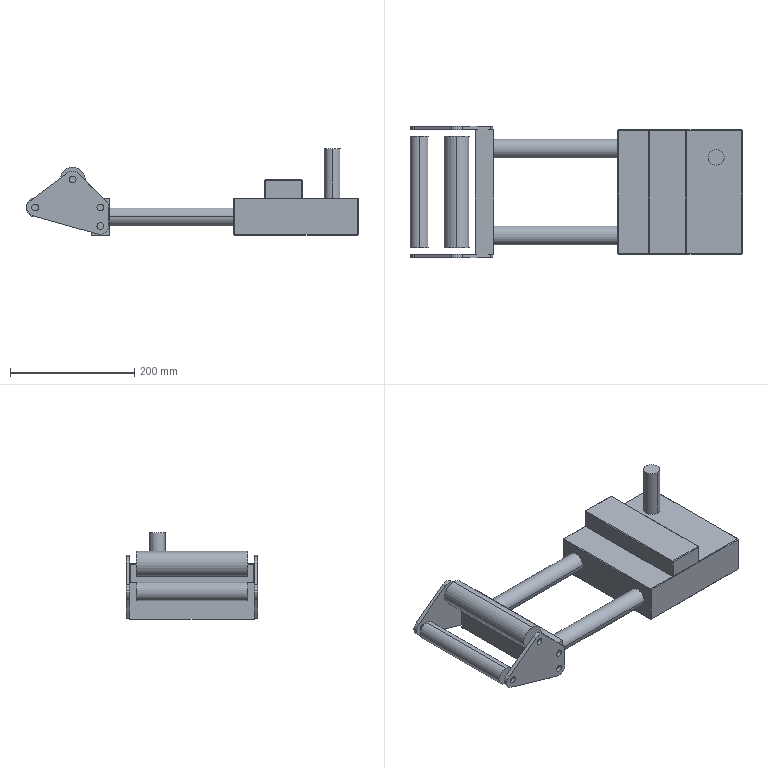Part | Creo | features PROTRUSION 8, CURVE 7, DATUM PLANE 3, CHAMFER 2, COORDINATE SYSTEM 1, MIRROR 1 | 3 solids | 95 faces | box 534.884 x 212 x 140 mm | volume 3889632 mm3 | plane 61 | cylinder 34 | commonest cylinder face diameters 11 x16 27.065 x8 30 x4 25.833 x2 29.768 x2 40 x2